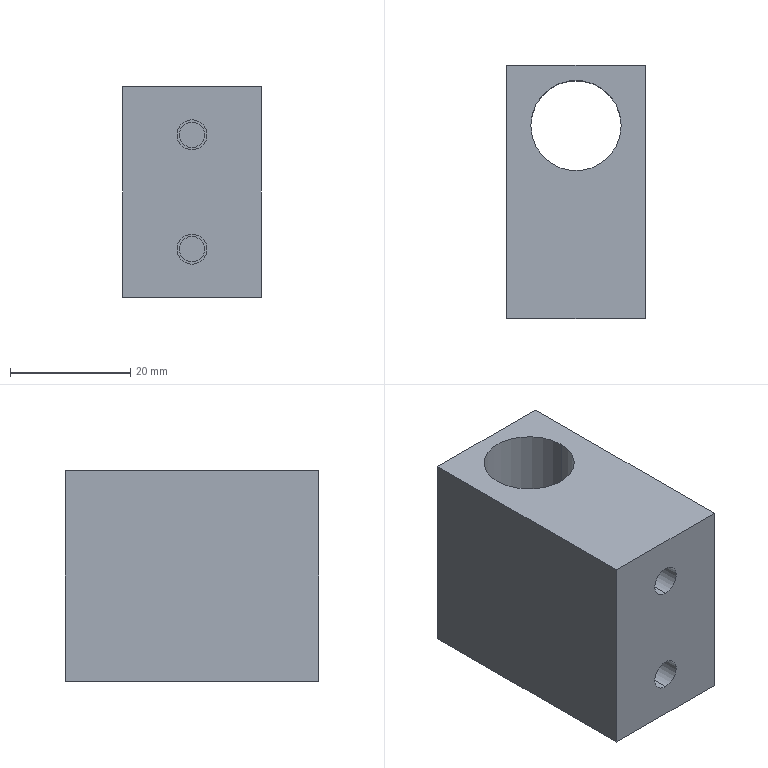Part | SolidWorks | features ICE 2, Extrusion 1 | 1 solid | 20 faces | box 23 x 42 x 35 mm | volume 27191 mm3 | cylinder 10 | plane 10 | commonest cylinder face diameters 4.2 x4 5 x4 15 x2
STEP:
#1=CARTESIAN_POINT('',(1.113,-7.744,10.1));
#2=VERTEX_POINT('',#1);
#3=CARTESIAN_POINT('',(1.113,-7.744,5.9));
#4=VERTEX_POINT('',#3);
#5=CARTESIAN_POINT('',(1.113,-7.744,8.));
#6=DIRECTION('',(0.,-1.,0.));
#7=DIRECTION('',(0.,0.,-1.));
#8=AXIS2_PLACEMENT_3D('',#5,#6,#7);
#9=CIRCLE('',#8,2.1);
#10=EDGE_CURVE('',#2,#4,#9,.T.);
#11=ORIENTED_EDGE('',*,*,#10,.F.);
#12=CARTESIAN_POINT('',(1.113,-9.244,10.1));
#13=VERTEX_POINT('',#12);
#14=CARTESIAN_POINT('',(1.113,-7.744,10.1));
#15=DIRECTION('',(0.,-1.,0.));
#16=VECTOR('',#15,1000.);
#17=LINE('',#14,#16);
#18=EDGE_CURVE('',#2,#13,#17,.T.);
#19=ORIENTED_EDGE('',*,*,#18,.T.);
#20=CARTESIAN_POINT('',(1.113,-9.244,5.9));
#21=VERTEX_POINT('',#20);
#22=CARTESIAN_POINT('',(1.113,-9.244,8.));
#23=DIRECTION('',(0.,1.,0.));
#24=DIRECTION('',(0.,0.,-1.));
#25=AXIS2_PLACEMENT_3D('',#22,#23,#24);
#26=CIRCLE('',#25,2.1);
#27=EDGE_CURVE('',#21,#13,#26,.T.);
#28=ORIENTED_EDGE('',*,*,#27,.F.);
#29=CARTESIAN_POINT('',(1.113,-7.744,5.9));
#30=DIRECTION('',(0.,-1.,0.));
#31=VECTOR('',#30,1000.);
#32=LINE('',#29,#31);
#33=EDGE_CURVE('',#4,#21,#32,.T.);
#34=ORIENTED_EDGE('',*,*,#33,.F.);
#35=EDGE_LOOP('',(#11,#19,#28,#34));
#36=FACE_OUTER_BOUND('',#35,.T.);
#37=CARTESIAN_POINT('',(1.113,-7.744,8.));
#38=DIRECTION('',(0.,-1.,0.));
#39=DIRECTION('',(0.,0.,-1.));
#40=AXIS2_PLACEMENT_3D('',#37,#38,#39);
#41=CYLINDRICAL_SURFACE('',#40,2.1);
#42=ADVANCED_FACE('',(#36),#41,.F.);
#43=CARTESIAN_POINT('',(1.113,-7.744,29.1));
#44=VERTEX_POINT('',#43);
#45=CARTESIAN_POINT('',(1.113,-7.744,24.9));
#46=VERTEX_POINT('',#45);
#47=CARTESIAN_POINT('',(1.113,-7.744,27.));
#48=DIRECTION('',(0.,-1.,0.));
#49=DIRECTION('',(0.,0.,-1.));
#50=AXIS2_PLACEMENT_3D('',#47,#48,#49);
#51=CIRCLE('',#50,2.1);
#52=EDGE_CURVE('',#44,#46,#51,.T.);
#53=ORIENTED_EDGE('',*,*,#52,.F.);
#54=CARTESIAN_POINT('',(1.113,-9.244,29.1));
#55=VERTEX_POINT('',#54);
#56=CARTESIAN_POINT('',(1.113,-7.744,29.1));
#57=DIRECTION('',(0.,-1.,0.));
#58=VECTOR('',#57,1000.);
#59=LINE('',#56,#58);
#60=EDGE_CURVE('',#44,#55,#59,.T.);
#61=ORIENTED_EDGE('',*,*,#60,.T.);
#62=CARTESIAN_POINT('',(1.113,-9.244,24.9));
#63=VERTEX_POINT('',#62);
#64=CARTESIAN_POINT('',(1.113,-9.244,27.));
#65=DIRECTION('',(0.,1.,0.));
#66=DIRECTION('',(0.,0.,-1.));
#67=AXIS2_PLACEMENT_3D('',#64,#65,#66);
#68=CIRCLE('',#67,2.1);
#69=EDGE_CURVE('',#63,#55,#68,.T.);
#70=ORIENTED_EDGE('',*,*,#69,.F.);
#71=CARTESIAN_POINT('',(1.113,-7.744,24.9));
#72=DIRECTION('',(0.,-1.,0.));
#73=VECTOR('',#72,1000.);
#74=LINE('',#71,#73);
#75=EDGE_CURVE('',#46,#63,#74,.T.);
#76=ORIENTED_EDGE('',*,*,#75,.F.);
#77=EDGE_LOOP('',(#53,#61,#70,#76));
#78=FACE_OUTER_BOUND('',#77,.T.);
#79=CARTESIAN_POINT('',(1.113,-7.744,27.));
#80=DIRECTION('',(0.,-1.,0.));
#81=DIRECTION('',(0.,0.,-1.));
#82=AXIS2_PLACEMENT_3D('',#79,#80,#81);
#83=CYLINDRICAL_SURFACE('',#82,2.1);
#84=ADVANCED_FACE('',(#78),#83,.F.);
#85=CARTESIAN_POINT('',(1.113,-9.244,10.5));
#86=VERTEX_POINT('',#85);
#87=CARTESIAN_POINT('',(1.113,-9.244,5.5));
#88=VERTEX_POINT('',#87);
#89=CARTESIAN_POINT('',(1.113,-9.244,8.));
#90=DIRECTION('',(0.,-1.,0.));
#91=DIRECTION('',(0.,0.,-1.));
#92=AXIS2_PLACEMENT_3D('',#89,#90,#91);
#93=CIRCLE('',#92,2.5);
#94=EDGE_CURVE('',#86,#88,#93,.T.);
#95=ORIENTED_EDGE('',*,*,#94,.F.);
#96=CARTESIAN_POINT('',(1.113,-19.244,10.5));
#97=VERTEX_POINT('',#96);
#98=CARTESIAN_POINT('',(1.113,-9.244,10.5));
#99=DIRECTION('',(0.,-1.,0.));
#100=VECTOR('',#99,1000.);
#101=LINE('',#98,#100);
#102=EDGE_CURVE('',#86,#97,#101,.T.);
#103=ORIENTED_EDGE('',*,*,#102,.T.);
#104=CARTESIAN_POINT('',(1.113,-19.244,5.5));
#105=VERTEX_POINT('',#104);
#106=CARTESIAN_POINT('',(1.113,-19.244,8.));
#107=DIRECTION('',(0.,-1.,0.));
#108=DIRECTION('',(0.,0.,-1.));
#109=AXIS2_PLACEMENT_3D('',#106,#107,#108);
#110=CIRCLE('',#109,2.5);
#111=EDGE_CURVE('',#97,#105,#110,.T.);
#112=ORIENTED_EDGE('',*,*,#111,.T.);
#113=CARTESIAN_POINT('',(1.113,-9.244,5.5));
#114=DIRECTION('',(0.,-1.,0.));
#115=VECTOR('',#114,1000.);
#116=LINE('',#113,#115);
#117=EDGE_CURVE('',#88,#105,#116,.T.);
#118=ORIENTED_EDGE('',*,*,#117,.F.);
#119=EDGE_LOOP('',(#95,#103,#112,#118));
#120=FACE_OUTER_BOUND('',#119,.T.);
#121=CARTESIAN_POINT('',(1.113,-9.244,8.));
#122=DIRECTION('',(0.,-1.,0.));
#123=DIRECTION('',(0.,0.,-1.));
#124=AXIS2_PLACEMENT_3D('',#121,#122,#123);
#125=CYLINDRICAL_SURFACE('',#124,2.5);
#126=ADVANCED_FACE('',(#120),#125,.F.);
#127=CARTESIAN_POINT('',(1.113,-9.244,29.5));
#128=VERTEX_POINT('',#127);
#129=CARTESIAN_POINT('',(1.113,-9.244,24.5));
#130=VERTEX_POINT('',#129);
#131=CARTESIAN_POINT('',(1.113,-9.244,27.));
#132=DIRECTION('',(0.,-1.,0.));
#133=DIRECTION('',(0.,0.,-1.));
#134=AXIS2_PLACEMENT_3D('',#131,#132,#133);
#135=CIRCLE('',#134,2.5);
#136=EDGE_CURVE('',#128,#130,#135,.T.);
#137=ORIENTED_EDGE('',*,*,#136,.F.);
#138=CARTESIAN_POINT('',(1.113,-19.244,29.5));
#139=VERTEX_POINT('',#138);
#140=CARTESIAN_POINT('',(1.113,-9.244,29.5));
#141=DIRECTION('',(0.,-1.,0.));
#142=VECTOR('',#141,1000.);
#143=LINE('',#140,#142);
#144=EDGE_CURVE('',#128,#139,#143,.T.);
#145=ORIENTED_EDGE('',*,*,#144,.T.);
#146=CARTESIAN_POINT('',(1.113,-19.244,24.5));
#147=VERTEX_POINT('',#146);
#148=CARTESIAN_POINT('',(1.113,-19.244,27.));
#149=DIRECTION('',(0.,-1.,0.));
#150=DIRECTION('',(0.,0.,-1.));
#151=AXIS2_PLACEMENT_3D('',#148,#149,#150);
#152=CIRCLE('',#151,2.5);
#153=EDGE_CURVE('',#139,#147,#152,.T.);
#154=ORIENTED_EDGE('',*,*,#153,.T.);
#155=CARTESIAN_POINT('',(1.113,-9.244,24.5));
#156=DIRECTION('',(0.,-1.,0.));
#157=VECTOR('',#156,1000.);
#158=LINE('',#155,#157);
#159=EDGE_CURVE('',#130,#147,#158,.T.);
#160=ORIENTED_EDGE('',*,*,#159,.F.);
#161=EDGE_LOOP('',(#137,#145,#154,#160));
#162=FACE_OUTER_BOUND('',#161,.T.);
#163=CARTESIAN_POINT('',(1.113,-9.244,27.));
#164=DIRECTION('',(0.,-1.,0.));
#165=DIRECTION('',(0.,0.,-1.));
#166=AXIS2_PLACEMENT_3D('',#163,#164,#165);
#167=CYLINDRICAL_SURFACE('',#166,2.5);
#168=ADVANCED_FACE('',(#162),#167,.F.);
#169=CARTESIAN_POINT('',(-6.387,12.756,35.));
#170=VERTEX_POINT('',#169);
#171=CARTESIAN_POINT('',(8.613,12.756,35.));
#172=VERTEX_POINT('',#171);
#173=CARTESIAN_POINT('',(1.113,12.756,35.));
#174=DIRECTION('',(0.,0.,1.));
#175=DIRECTION('',(1.,0.,0.));
#176=AXIS2_PLACEMENT_3D('',#173,#174,#175);
#177=CIRCLE('',#176,7.5);
#178=EDGE_CURVE('',#170,#172,#177,.T.);
#179=ORIENTED_EDGE('',*,*,#178,.T.);
#180=CARTESIAN_POINT('',(8.613,12.756,0.));
#181=VERTEX_POINT('',#180);
#182=CARTESIAN_POINT('',(8.613,12.756,35.));
#183=DIRECTION('',(0.,0.,-1.));
#184=VECTOR('',#183,1000.);
#185=LINE('',#182,#184);
#186=EDGE_CURVE('',#172,#181,#185,.T.);
#187=ORIENTED_EDGE('',*,*,#186,.T.);
#188=CARTESIAN_POINT('',(-6.387,12.756,0.));
#189=VERTEX_POINT('',#188);
#190=CARTESIAN_POINT('',(1.113,12.756,0.));
#191=DIRECTION('',(0.,0.,1.));
#192=DIRECTION('',(1.,0.,0.));
#193=AXIS2_PLACEMENT_3D('',#190,#191,#192);
#194=CIRCLE('',#193,7.5);
#195=EDGE_CURVE('',#189,#181,#194,.T.);
#196=ORIENTED_EDGE('',*,*,#195,.F.);
#197=CARTESIAN_POINT('',(-6.387,12.756,35.));
#198=DIRECTION('',(0.,0.,-1.));
#199=VECTOR('',#198,1000.);
#200=LINE('',#197,#199);
#201=EDGE_CURVE('',#170,#189,#200,.T.);
#202=ORIENTED_EDGE('',*,*,#201,.F.);
#203=EDGE_LOOP('',(#179,#187,#196,#202));
#204=FACE_OUTER_BOUND('',#203,.T.);
#205=CARTESIAN_POINT('',(1.113,12.756,35.));
#206=DIRECTION('',(0.,0.,-1.));
#207=DIRECTION('',(-1.,0.,0.));
#208=AXIS2_PLACEMENT_3D('',#205,#206,#207);
#209=CYLINDRICAL_SURFACE('',#208,7.5);
#210=ADVANCED_FACE('',(#204),#209,.F.);
#211=CARTESIAN_POINT('',(-10.387,22.756,35.));
#212=VERTEX_POINT('',#211);
#213=CARTESIAN_POINT('',(-10.387,-19.244,35.));
#214=VERTEX_POINT('',#213);
#215=CARTESIAN_POINT('',(-10.387,22.756,35.));
#216=DIRECTION('',(0.,-1.,0.));
#217=VECTOR('',#216,1000.);
#218=LINE('',#215,#217);
#219=EDGE_CURVE('',#212,#214,#218,.T.);
#220=ORIENTED_EDGE('',*,*,#219,.T.);
#221=CARTESIAN_POINT('',(12.613,-19.244,35.));
#222=VERTEX_POINT('',#221);
#223=CARTESIAN_POINT('',(-10.387,-19.244,35.));
#224=DIRECTION('',(1.,0.,0.));
#225=VECTOR('',#224,1000.);
#226=LINE('',#223,#225);
#227=EDGE_CURVE('',#214,#222,#226,.T.);
#228=ORIENTED_EDGE('',*,*,#227,.T.);
#229=CARTESIAN_POINT('',(12.613,22.756,35.));
#230=VERTEX_POINT('',#229);
#231=CARTESIAN_POINT('',(12.613,22.756,35.));
#232=DIRECTION('',(0.,1.,0.));
#233=VECTOR('',#232,1000.);
#234=LINE('',#231,#233);
#235=EDGE_CURVE('',#222,#230,#234,.T.);
#236=ORIENTED_EDGE('',*,*,#235,.T.);
#237=CARTESIAN_POINT('',(-10.387,22.756,35.));
#238=DIRECTION('',(-1.,0.,0.));
#239=VECTOR('',#238,1000.);
#240=LINE('',#237,#239);
#241=EDGE_CURVE('',#230,#212,#240,.T.);
#242=ORIENTED_EDGE('',*,*,#241,.T.);
#243=EDGE_LOOP('',(#220,#228,#236,#242));
#244=FACE_OUTER_BOUND('',#243,.T.);
#245=ORIENTED_EDGE('',*,*,#178,.F.);
#246=CARTESIAN_POINT('',(1.113,12.756,35.));
#247=DIRECTION('',(0.,0.,1.));
#248=DIRECTION('',(1.,0.,0.));
#249=AXIS2_PLACEMENT_3D('',#246,#247,#248);
#250=CIRCLE('',#249,7.5);
#251=EDGE_CURVE('',#172,#170,#250,.T.);
#252=ORIENTED_EDGE('',*,*,#251,.F.);
#253=EDGE_LOOP('',(#245,#252));
#254=FACE_BOUND('',#253,.T.);
#255=CARTESIAN_POINT('',(0.,0.,35.));
#256=DIRECTION('',(0.,0.,1.));
#257=DIRECTION('',(1.,0.,0.));
#258=AXIS2_PLACEMENT_3D('',#255,#256,#257);
#259=PLANE('',#258);
#260=ADVANCED_FACE('',(#244,#254),#259,.T.);
#261=CARTESIAN_POINT('',(-10.387,22.756,0.));
#262=VERTEX_POINT('',#261);
#263=CARTESIAN_POINT('',(-10.387,-19.244,0.));
#264=VERTEX_POINT('',#263);
#265=CARTESIAN_POINT('',(-10.387,22.756,0.));
#266=DIRECTION('',(0.,-1.,0.));
#267=VECTOR('',#266,1000.);
#268=LINE('',#265,#267);
#269=EDGE_CURVE('',#262,#264,#268,.T.);
#270=ORIENTED_EDGE('',*,*,#269,.F.);
#271=CARTESIAN_POINT('',(12.613,22.756,0.));
#272=VERTEX_POINT('',#271);
#273=CARTESIAN_POINT('',(-10.387,22.756,0.));
#274=DIRECTION('',(-1.,0.,0.));
#275=VECTOR('',#274,1000.);
#276=LINE('',#273,#275);
#277=EDGE_CURVE('',#272,#262,#276,.T.);
#278=ORIENTED_EDGE('',*,*,#277,.F.);
#279=CARTESIAN_POINT('',(12.613,-19.244,0.));
#280=VERTEX_POINT('',#279);
#281=CARTESIAN_POINT('',(12.613,22.756,0.));
#282=DIRECTION('',(0.,1.,0.));
#283=VECTOR('',#282,1000.);
#284=LINE('',#281,#283);
#285=EDGE_CURVE('',#280,#272,#284,.T.);
#286=ORIENTED_EDGE('',*,*,#285,.F.);
#287=CARTESIAN_POINT('',(-10.387,-19.244,0.));
#288=DIRECTION('',(1.,0.,0.));
#289=VECTOR('',#288,1000.);
#290=LINE('',#287,#289);
#291=EDGE_CURVE('',#264,#280,#290,.T.);
#292=ORIENTED_EDGE('',*,*,#291,.F.);
#293=EDGE_LOOP('',(#270,#278,#286,#292));
#294=FACE_OUTER_BOUND('',#293,.T.);
#295=ORIENTED_EDGE('',*,*,#195,.T.);
#296=CARTESIAN_POINT('',(1.113,12.756,0.));
#297=DIRECTION('',(0.,0.,1.));
#298=DIRECTION('',(1.,0.,0.));
#299=AXIS2_PLACEMENT_3D('',#296,#297,#298);
#300=CIRCLE('',#299,7.5);
#301=EDGE_CURVE('',#181,#189,#300,.T.);
#302=ORIENTED_EDGE('',*,*,#301,.T.);
#303=EDGE_LOOP('',(#295,#302));
#304=FACE_BOUND('',#303,.T.);
#305=CARTESIAN_POINT('',(0.,0.,0.));
#306=DIRECTION('',(0.,0.,1.));
#307=DIRECTION('',(1.,0.,0.));
#308=AXIS2_PLACEMENT_3D('',#305,#306,#307);
#309=PLANE('',#308);
#310=ADVANCED_FACE('',(#294,#304),#309,.F.);
#311=ORIENTED_EDGE('',*,*,#269,.T.);
#312=CARTESIAN_POINT('',(-10.387,-19.244,35.));
#313=DIRECTION('',(0.,0.,-1.));
#314=VECTOR('',#313,1000.);
#315=LINE('',#312,#314);
#316=EDGE_CURVE('',#214,#264,#315,.T.);
#317=ORIENTED_EDGE('',*,*,#316,.F.);
#318=ORIENTED_EDGE('',*,*,#219,.F.);
#319=CARTESIAN_POINT('',(-10.387,22.756,35.));
#320=DIRECTION('',(0.,0.,-1.));
#321=VECTOR('',#320,1000.);
#322=LINE('',#319,#321);
#323=EDGE_CURVE('',#212,#262,#322,.T.);
#324=ORIENTED_EDGE('',*,*,#323,.T.);
#325=EDGE_LOOP('',(#311,#317,#318,#324));
#326=FACE_OUTER_BOUND('',#325,.T.);
#327=CARTESIAN_POINT('',(-10.387,22.756,35.));
#328=DIRECTION('',(1.,0.,0.));
#329=DIRECTION('',(0.,1.,0.));
#330=AXIS2_PLACEMENT_3D('',#327,#328,#329);
#331=PLANE('',#330);
#332=ADVANCED_FACE('',(#326),#331,.F.);
#333=CARTESIAN_POINT('',(1.113,-19.244,27.));
#334=DIRECTION('',(0.,-1.,0.));
#335=DIRECTION('',(0.,0.,-1.));
#336=AXIS2_PLACEMENT_3D('',#333,#334,#335);
#337=CIRCLE('',#336,2.5);
#338=EDGE_CURVE('',#147,#139,#337,.T.);
#339=ORIENTED_EDGE('',*,*,#338,.F.);
#340=ORIENTED_EDGE('',*,*,#153,.F.);
#341=EDGE_LOOP('',(#339,#340));
#342=FACE_BOUND('',#341,.T.);
#343=CARTESIAN_POINT('',(1.113,-19.244,8.));
#344=DIRECTION('',(0.,-1.,0.));
#345=DIRECTION('',(0.,0.,-1.));
#346=AXIS2_PLACEMENT_3D('',#343,#344,#345);
#347=CIRCLE('',#346,2.5);
#348=EDGE_CURVE('',#105,#97,#347,.T.);
#349=ORIENTED_EDGE('',*,*,#348,.F.);
#350=ORIENTED_EDGE('',*,*,#111,.F.);
#351=EDGE_LOOP('',(#349,#350));
#352=FACE_BOUND('',#351,.T.);
#353=ORIENTED_EDGE('',*,*,#291,.T.);
#354=CARTESIAN_POINT('',(12.613,-19.244,35.));
#355=DIRECTION('',(0.,0.,-1.));
#356=VECTOR('',#355,1000.);
#357=LINE('',#354,#356);
#358=EDGE_CURVE('',#222,#280,#357,.T.);
#359=ORIENTED_EDGE('',*,*,#358,.F.);
#360=ORIENTED_EDGE('',*,*,#227,.F.);
#361=ORIENTED_EDGE('',*,*,#316,.T.);
#362=EDGE_LOOP('',(#353,#359,#360,#361));
#363=FACE_OUTER_BOUND('',#362,.T.);
#364=CARTESIAN_POINT('',(-10.387,-19.244,35.));
#365=DIRECTION('',(0.,1.,0.));
#366=DIRECTION('',(0.,0.,1.));
#367=AXIS2_PLACEMENT_3D('',#364,#365,#366);
#368=PLANE('',#367);
#369=ADVANCED_FACE('',(#342,#352,#363),#368,.F.);
#370=ORIENTED_EDGE('',*,*,#285,.T.);
#371=CARTESIAN_POINT('',(12.613,22.756,35.));
#372=DIRECTION('',(0.,0.,-1.));
#373=VECTOR('',#372,1000.);
#374=LINE('',#371,#373);
#375=EDGE_CURVE('',#230,#272,#374,.T.);
#376=ORIENTED_EDGE('',*,*,#375,.F.);
#377=ORIENTED_EDGE('',*,*,#235,.F.);
#378=ORIENTED_EDGE('',*,*,#358,.T.);
#379=EDGE_LOOP('',(#370,#376,#377,#378));
#380=FACE_OUTER_BOUND('',#379,.T.);
#381=CARTESIAN_POINT('',(12.613,22.756,35.));
#382=DIRECTION('',(-1.,0.,0.));
#383=DIRECTION('',(0.,-1.,0.));
#384=AXIS2_PLACEMENT_3D('',#381,#382,#383);
#385=PLANE('',#384);
#386=ADVANCED_FACE('',(#380),#385,.F.);
#387=ORIENTED_EDGE('',*,*,#277,.T.);
#388=ORIENTED_EDGE('',*,*,#323,.F.);
#389=ORIENTED_EDGE('',*,*,#241,.F.);
#390=ORIENTED_EDGE('',*,*,#375,.T.);
#391=EDGE_LOOP('',(#387,#388,#389,#390));
#392=FACE_OUTER_BOUND('',#391,.T.);
#393=CARTESIAN_POINT('',(-10.387,22.756,35.));
#394=DIRECTION('',(0.,-1.,0.));
#395=DIRECTION('',(0.,0.,-1.));
#396=AXIS2_PLACEMENT_3D('',#393,#394,#395);
#397=PLANE('',#396);
#398=ADVANCED_FACE('',(#392),#397,.F.);
#399=ORIENTED_EDGE('',*,*,#186,.F.);
#400=ORIENTED_EDGE('',*,*,#251,.T.);
#401=ORIENTED_EDGE('',*,*,#201,.T.);
#402=ORIENTED_EDGE('',*,*,#301,.F.);
#403=EDGE_LOOP('',(#399,#400,#401,#402));
#404=FACE_OUTER_BOUND('',#403,.T.);
#405=CARTESIAN_POINT('',(1.113,12.756,35.));
#406=DIRECTION('',(0.,0.,-1.));
#407=DIRECTION('',(-1.,0.,0.));
#408=AXIS2_PLACEMENT_3D('',#405,#406,#407);
#409=CYLINDRICAL_SURFACE('',#408,7.5);
#410=ADVANCED_FACE('',(#404),#409,.F.);
#411=CARTESIAN_POINT('',(1.113,-9.244,27.));
#412=DIRECTION('',(0.,-1.,0.));
#413=DIRECTION('',(0.,0.,-1.));
#414=AXIS2_PLACEMENT_3D('',#411,#412,#413);
#415=CIRCLE('',#414,2.5);
#416=EDGE_CURVE('',#130,#128,#415,.T.);
#417=ORIENTED_EDGE('',*,*,#416,.T.);
#418=ORIENTED_EDGE('',*,*,#136,.T.);
#419=EDGE_LOOP('',(#417,#418));
#420=FACE_OUTER_BOUND('',#419,.T.);
#421=ORIENTED_EDGE('',*,*,#69,.T.);
#422=CARTESIAN_POINT('',(1.113,-9.244,27.));
#423=DIRECTION('',(0.,1.,0.));
#424=DIRECTION('',(0.,0.,-1.));
#425=AXIS2_PLACEMENT_3D('',#422,#423,#424);
#426=CIRCLE('',#425,2.1);
#427=EDGE_CURVE('',#55,#63,#426,.T.);
#428=ORIENTED_EDGE('',*,*,#427,.T.);
#429=EDGE_LOOP('',(#421,#428));
#430=FACE_BOUND('',#429,.T.);
#431=CARTESIAN_POINT('',(1.113,-9.244,27.));
#432=DIRECTION('',(0.,-1.,0.));
#433=DIRECTION('',(0.,0.,-1.));
#434=AXIS2_PLACEMENT_3D('',#431,#432,#433);
#435=PLANE('',#434);
#436=ADVANCED_FACE('',(#420,#430),#435,.T.);
#437=ORIENTED_EDGE('',*,*,#144,.F.);
#438=ORIENTED_EDGE('',*,*,#416,.F.);
#439=ORIENTED_EDGE('',*,*,#159,.T.);
#440=ORIENTED_EDGE('',*,*,#338,.T.);
#441=EDGE_LOOP('',(#437,#438,#439,#440));
#442=FACE_OUTER_BOUND('',#441,.T.);
#443=CARTESIAN_POINT('',(1.113,-9.244,27.));
#444=DIRECTION('',(0.,-1.,0.));
#445=DIRECTION('',(0.,0.,-1.));
#446=AXIS2_PLACEMENT_3D('',#443,#444,#445);
#447=CYLINDRICAL_SURFACE('',#446,2.5);
#448=ADVANCED_FACE('',(#442),#447,.F.);
#449=CARTESIAN_POINT('',(1.113,-9.244,8.));
#450=DIRECTION('',(0.,-1.,0.));
#451=DIRECTION('',(0.,0.,-1.));
#452=AXIS2_PLACEMENT_3D('',#449,#450,#451);
#453=CIRCLE('',#452,2.5);
#454=EDGE_CURVE('',#88,#86,#453,.T.);
#455=ORIENTED_EDGE('',*,*,#454,.T.);
#456=ORIENTED_EDGE('',*,*,#94,.T.);
#457=EDGE_LOOP('',(#455,#456));
#458=FACE_OUTER_BOUND('',#457,.T.);
#459=ORIENTED_EDGE('',*,*,#27,.T.);
#460=CARTESIAN_POINT('',(1.113,-9.244,8.));
#461=DIRECTION('',(0.,1.,0.));
#462=DIRECTION('',(0.,0.,-1.));
#463=AXIS2_PLACEMENT_3D('',#460,#461,#462);
#464=CIRCLE('',#463,2.1);
#465=EDGE_CURVE('',#13,#21,#464,.T.);
#466=ORIENTED_EDGE('',*,*,#465,.T.);
#467=EDGE_LOOP('',(#459,#466));
#468=FACE_BOUND('',#467,.T.);
#469=CARTESIAN_POINT('',(1.113,-9.244,8.));
#470=DIRECTION('',(0.,-1.,0.));
#471=DIRECTION('',(0.,0.,-1.));
#472=AXIS2_PLACEMENT_3D('',#469,#470,#471);
#473=PLANE('',#472);
#474=ADVANCED_FACE('',(#458,#468),#473,.T.);
#475=ORIENTED_EDGE('',*,*,#102,.F.);
#476=ORIENTED_EDGE('',*,*,#454,.F.);
#477=ORIENTED_EDGE('',*,*,#117,.T.);
#478=ORIENTED_EDGE('',*,*,#348,.T.);
#479=EDGE_LOOP('',(#475,#476,#477,#478));
#480=FACE_OUTER_BOUND('',#479,.T.);
#481=CARTESIAN_POINT('',(1.113,-9.244,8.));
#482=DIRECTION('',(0.,-1.,0.));
#483=DIRECTION('',(0.,0.,-1.));
#484=AXIS2_PLACEMENT_3D('',#481,#482,#483);
#485=CYLINDRICAL_SURFACE('',#484,2.5);
#486=ADVANCED_FACE('',(#480),#485,.F.);
#487=CARTESIAN_POINT('',(1.113,-7.744,27.));
#488=DIRECTION('',(0.,-1.,0.));
#489=DIRECTION('',(0.,0.,-1.));
#490=AXIS2_PLACEMENT_3D('',#487,#488,#489);
#491=CIRCLE('',#490,2.1);
#492=EDGE_CURVE('',#46,#44,#491,.T.);
#493=ORIENTED_EDGE('',*,*,#492,.T.);
#494=ORIENTED_EDGE('',*,*,#52,.T.);
#495=EDGE_LOOP('',(#493,#494));
#496=FACE_OUTER_BOUND('',#495,.T.);
#497=CARTESIAN_POINT('',(1.113,-7.744,27.));
#498=DIRECTION('',(0.,-1.,0.));
#499=DIRECTION('',(0.,0.,-1.));
#500=AXIS2_PLACEMENT_3D('',#497,#498,#499);
#501=PLANE('',#500);
#502=ADVANCED_FACE('',(#496),#501,.T.);
#503=ORIENTED_EDGE('',*,*,#60,.F.);
#504=ORIENTED_EDGE('',*,*,#492,.F.);
#505=ORIENTED_EDGE('',*,*,#75,.T.);
#506=ORIENTED_EDGE('',*,*,#427,.F.);
#507=EDGE_LOOP('',(#503,#504,#505,#506));
#508=FACE_OUTER_BOUND('',#507,.T.);
#509=CARTESIAN_POINT('',(1.113,-7.744,27.));
#510=DIRECTION('',(0.,-1.,0.));
#511=DIRECTION('',(0.,0.,-1.));
#512=AXIS2_PLACEMENT_3D('',#509,#510,#511);
#513=CYLINDRICAL_SURFACE('',#512,2.1);
#514=ADVANCED_FACE('',(#508),#513,.F.);
#515=CARTESIAN_POINT('',(1.113,-7.744,8.));
#516=DIRECTION('',(0.,-1.,0.));
#517=DIRECTION('',(0.,0.,-1.));
#518=AXIS2_PLACEMENT_3D('',#515,#516,#517);
#519=CIRCLE('',#518,2.1);
#520=EDGE_CURVE('',#4,#2,#519,.T.);
#521=ORIENTED_EDGE('',*,*,#520,.T.);
#522=ORIENTED_EDGE('',*,*,#10,.T.);
#523=EDGE_LOOP('',(#521,#522));
#524=FACE_OUTER_BOUND('',#523,.T.);
#525=CARTESIAN_POINT('',(1.113,-7.744,8.));
#526=DIRECTION('',(0.,-1.,0.));
#527=DIRECTION('',(0.,0.,-1.));
#528=AXIS2_PLACEMENT_3D('',#525,#526,#527);
#529=PLANE('',#528);
#530=ADVANCED_FACE('',(#524),#529,.T.);
#531=ORIENTED_EDGE('',*,*,#18,.F.);
#532=ORIENTED_EDGE('',*,*,#520,.F.);
#533=ORIENTED_EDGE('',*,*,#33,.T.);
#534=ORIENTED_EDGE('',*,*,#465,.F.);
#535=EDGE_LOOP('',(#531,#532,#533,#534));
#536=FACE_OUTER_BOUND('',#535,.T.);
#537=CARTESIAN_POINT('',(1.113,-7.744,8.));
#538=DIRECTION('',(0.,-1.,0.));
#539=DIRECTION('',(0.,0.,-1.));
#540=AXIS2_PLACEMENT_3D('',#537,#538,#539);
#541=CYLINDRICAL_SURFACE('',#540,2.1);
#542=ADVANCED_FACE('',(#536),#541,.F.);
#543=CLOSED_SHELL('',(#42,#84,#126,#168,#210,#260,#310,#332,#369,#386,#398,#410,#436,#448,#474,#486,#502,#514,#530,#542));
#544=MANIFOLD_SOLID_BREP('',#543);
#545=CARTESIAN_POINT('',(0.,0.,0.));
#546=DIRECTION('',(0.,0.,1.));
#547=DIRECTION('',(1.,0.,0.));
#548=AXIS2_PLACEMENT_3D('',#545,#546,#547);
#549=(LENGTH_UNIT()NAMED_UNIT(*)SI_UNIT(.MILLI.,.METRE.));
#550=UNCERTAINTY_MEASURE_WITH_UNIT(LENGTH_MEASURE(0.00001),#549,'','');
#551=(NAMED_UNIT(*)PLANE_ANGLE_UNIT()SI_UNIT($,.RADIAN.));
#552=(NAMED_UNIT(*)SI_UNIT($,.STERADIAN.)SOLID_ANGLE_UNIT());
#553=(GEOMETRIC_REPRESENTATION_CONTEXT(3)GLOBAL_UNCERTAINTY_ASSIGNED_CONTEXT((#550))GLOBAL_UNIT_ASSIGNED_CONTEXT((#549,#551,#552))REPRESENTATION_CONTEXT('',''));
#554=ADVANCED_BREP_SHAPE_REPRESENTATION('',(#544,#548),#553);